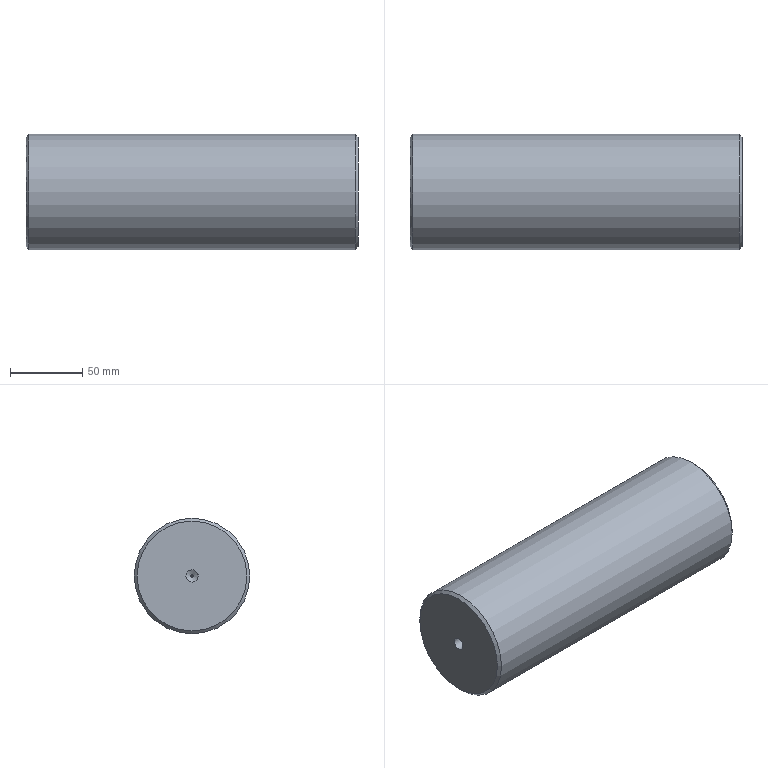Part | STEP file | solid 31 | 1 solid | 8 faces | box 230 x 80 x 80 mm | volume 1153880 mm3 | plane 3 | cone 3 | cylinder 2 | commonest cylinder face diameters 8.5 x1 80 x1